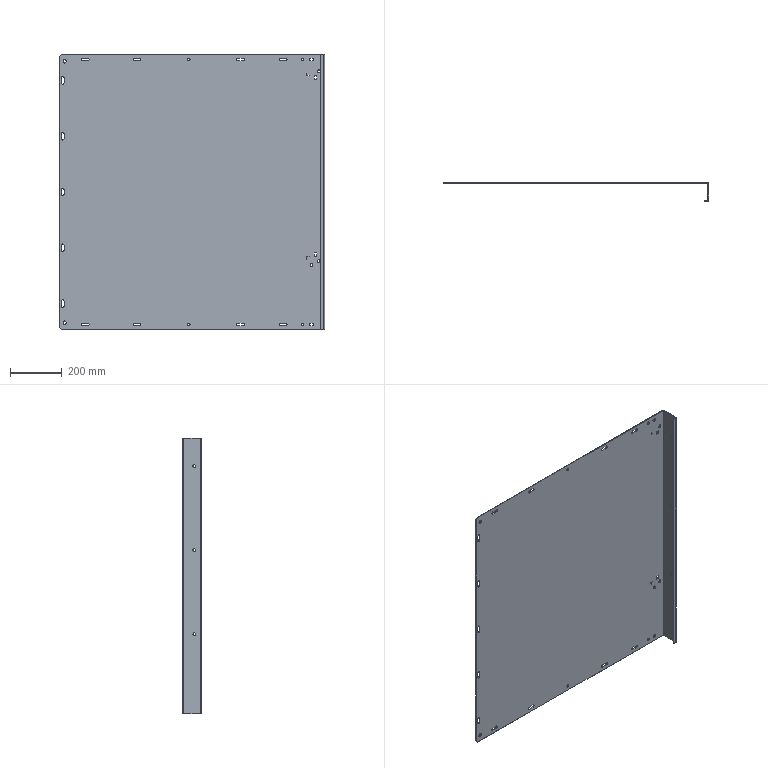Part | 1 solid | 133 faces | box 1025 x 72 x 1064 mm | volume 3509524 mm3 | plane 68 | cylinder 65 | commonest cylinder face diameters 10 x39 10.5 x12 11 x4 12.5 x4 0.4 x2 6.4 x2